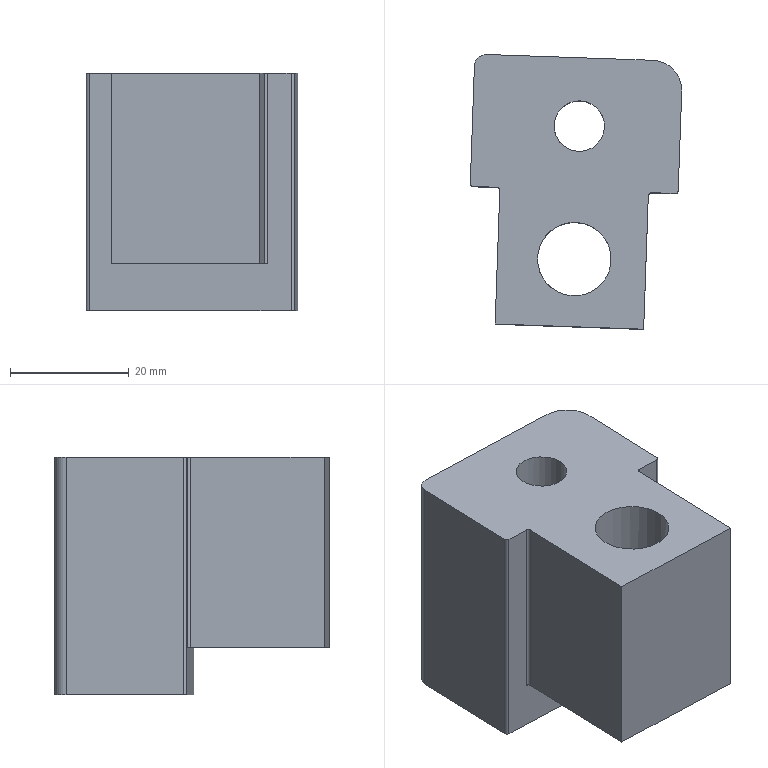Part | NX | features PS-21 2 | 1 solid | 20 faces | box 35.567 x 46.214 x 40 mm | volume 41123 mm3 | plane 11 | cylinder 9 | commonest cylinder face diameters 1 x4 4 x1 8.506 x1 10 x1 12.4 x1 14.5 x1
STEP:
#1=CARTESIAN_POINT('',(3099.937,-917.63,900.716));
#2=VERTEX_POINT('',#1);
#3=CARTESIAN_POINT('',(3100.722,-895.143,900.716));
#4=VERTEX_POINT('',#3);
#5=CARTESIAN_POINT('',(3098.831,-949.294,900.716));
#6=DIRECTION('',(-0.0349,-0.9994,0.));
#7=VECTOR('',#6,1000.);
#8=LINE('',#5,#7);
#9=EDGE_CURVE('',#2,#4,#8,.F.);
#10=ORIENTED_EDGE('',*,*,#9,.T.);
#11=CARTESIAN_POINT('',(3100.722,-895.143,868.716));
#12=VERTEX_POINT('',#11);
#13=CARTESIAN_POINT('',(3100.722,-895.143,868.716));
#14=DIRECTION('',(0.,0.,-1.));
#15=VECTOR('',#14,1000.);
#16=LINE('',#13,#15);
#17=EDGE_CURVE('',#4,#12,#16,.T.);
#18=ORIENTED_EDGE('',*,*,#17,.T.);
#19=CARTESIAN_POINT('',(3099.937,-917.63,868.716));
#20=VERTEX_POINT('',#19);
#21=CARTESIAN_POINT('',(3100.334,-906.255,868.716));
#22=DIRECTION('',(0.0349,0.9994,0.));
#23=VECTOR('',#22,1000.);
#24=LINE('',#21,#23);
#25=EDGE_CURVE('',#20,#12,#24,.T.);
#26=ORIENTED_EDGE('',*,*,#25,.F.);
#27=CARTESIAN_POINT('',(3099.937,-917.63,890.716));
#28=DIRECTION('',(0.,0.,1.));
#29=VECTOR('',#28,1000.);
#30=LINE('',#27,#29);
#31=EDGE_CURVE('',#2,#20,#30,.F.);
#32=ORIENTED_EDGE('',*,*,#31,.F.);
#33=EDGE_LOOP('',(#10,#18,#26,#32));
#34=FACE_BOUND('',#33,.T.);
#35=CARTESIAN_POINT('',(3100.52,-900.918,890.716));
#36=DIRECTION('',(0.9994,-0.0349,0.));
#37=DIRECTION('',(-0.0349,-0.9994,0.));
#38=AXIS2_PLACEMENT_3D('',#35,#36,#37);
#39=PLANE('',#38);
#40=ADVANCED_FACE('',(#34),#39,.F.);
#41=CARTESIAN_POINT('',(3124.922,-918.502,868.716));
#42=VERTEX_POINT('',#41);
#43=CARTESIAN_POINT('',(3109.742,-917.972,868.716));
#44=DIRECTION('',(0.9994,-0.0349,0.));
#45=VECTOR('',#44,1000.);
#46=LINE('',#43,#45);
#47=EDGE_CURVE('',#42,#20,#46,.F.);
#48=ORIENTED_EDGE('',*,*,#47,.F.);
#49=CARTESIAN_POINT('',(3124.922,-918.502,900.716));
#50=VERTEX_POINT('',#49);
#51=CARTESIAN_POINT('',(3124.922,-918.502,862.716));
#52=DIRECTION('',(0.,0.,1.));
#53=VECTOR('',#52,1000.);
#54=LINE('',#51,#53);
#55=EDGE_CURVE('',#50,#42,#54,.F.);
#56=ORIENTED_EDGE('',*,*,#55,.F.);
#57=CARTESIAN_POINT('',(3109.742,-917.972,900.716));
#58=DIRECTION('',(-0.9994,0.0349,0.));
#59=VECTOR('',#58,1000.);
#60=LINE('',#57,#59);
#61=EDGE_CURVE('',#50,#2,#60,.T.);
#62=ORIENTED_EDGE('',*,*,#61,.T.);
#63=ORIENTED_EDGE('',*,*,#31,.T.);
#64=EDGE_LOOP('',(#48,#56,#62,#63));
#65=FACE_BOUND('',#64,.T.);
#66=CARTESIAN_POINT('',(3109.742,-917.972,863.216));
#67=DIRECTION('',(0.0349,0.9994,0.));
#68=DIRECTION('',(-0.9994,0.0349,0.));
#69=AXIS2_PLACEMENT_3D('',#66,#67,#68);
#70=PLANE('',#69);
#71=ADVANCED_FACE('',(#65),#70,.F.);
#72=CARTESIAN_POINT('',(3125.707,-896.016,868.716));
#73=VERTEX_POINT('',#72);
#74=CARTESIAN_POINT('',(3125.319,-907.127,868.716));
#75=DIRECTION('',(0.0349,0.9994,0.));
#76=VECTOR('',#75,1000.);
#77=LINE('',#74,#76);
#78=EDGE_CURVE('',#42,#73,#77,.T.);
#79=ORIENTED_EDGE('',*,*,#78,.T.);
#80=CARTESIAN_POINT('',(3125.707,-896.016,900.716));
#81=VERTEX_POINT('',#80);
#82=CARTESIAN_POINT('',(3125.707,-896.016,862.716));
#83=DIRECTION('',(0.,0.,-1.));
#84=VECTOR('',#83,1000.);
#85=LINE('',#82,#84);
#86=EDGE_CURVE('',#73,#81,#85,.F.);
#87=ORIENTED_EDGE('',*,*,#86,.T.);
#88=CARTESIAN_POINT('',(3123.816,-950.166,900.716));
#89=DIRECTION('',(-0.0349,-0.9994,0.));
#90=VECTOR('',#89,1000.);
#91=LINE('',#88,#90);
#92=EDGE_CURVE('',#50,#81,#91,.F.);
#93=ORIENTED_EDGE('',*,*,#92,.F.);
#94=ORIENTED_EDGE('',*,*,#55,.T.);
#95=EDGE_LOOP('',(#79,#87,#93,#94));
#96=FACE_BOUND('',#95,.T.);
#97=CARTESIAN_POINT('',(3125.54,-900.791,862.716));
#98=DIRECTION('',(0.9994,-0.0349,0.));
#99=DIRECTION('',(-0.0349,-0.9994,0.));
#100=AXIS2_PLACEMENT_3D('',#97,#98,#99);
#101=PLANE('',#100);
#102=ADVANCED_FACE('',(#96),#101,.T.);
#103=CARTESIAN_POINT('',(3107.081,-906.274,868.716));
#104=VERTEX_POINT('',#103);
#105=CARTESIAN_POINT('',(3113.266,-906.707,868.716));
#106=DIRECTION('',(0.,0.,1.));
#107=DIRECTION('',(-0.9976,0.06975,0.));
#108=AXIS2_PLACEMENT_3D('',#105,#106,#107);
#109=CIRCLE('',#108,6.2);
#110=EDGE_CURVE('',#104,#104,#109,.T.);
#111=ORIENTED_EDGE('',*,*,#110,.F.);
#112=EDGE_LOOP('',(#111));
#113=FACE_BOUND('',#112,.T.);
#114=CARTESIAN_POINT('',(3113.266,-900.507,900.716));
#115=VERTEX_POINT('',#114);
#116=CARTESIAN_POINT('',(3113.266,-906.707,900.716));
#117=DIRECTION('',(0.,0.,-1.));
#118=DIRECTION('',(0.,1.,0.));
#119=AXIS2_PLACEMENT_3D('',#116,#117,#118);
#120=CIRCLE('',#119,6.2);
#121=EDGE_CURVE('',#115,#115,#120,.F.);
#122=ORIENTED_EDGE('',*,*,#121,.T.);
#123=EDGE_LOOP('',(#122));
#124=FACE_BOUND('',#123,.T.);
#125=CARTESIAN_POINT('',(3113.266,-906.707,935.716));
#126=DIRECTION('',(0.,0.,-1.));
#127=DIRECTION('',(0.9976,-0.06975,0.));
#128=AXIS2_PLACEMENT_3D('',#125,#126,#127);
#129=CYLINDRICAL_SURFACE('',#128,6.2);
#130=ADVANCED_FACE('',(#113,#124),#129,.F.);
#131=CARTESIAN_POINT('',(3100.24,-894.626,868.716));
#132=VERTEX_POINT('',#131);
#133=CARTESIAN_POINT('',(3126.224,-895.534,868.716));
#134=VERTEX_POINT('',#133);
#135=CARTESIAN_POINT('',(3113.671,-895.095,868.716));
#136=DIRECTION('',(0.9994,-0.0349,0.));
#137=VECTOR('',#136,1000.);
#138=LINE('',#135,#137);
#139=EDGE_CURVE('',#132,#134,#138,.T.);
#140=ORIENTED_EDGE('',*,*,#139,.T.);
#141=CARTESIAN_POINT('',(3126.206,-896.033,868.716));
#142=DIRECTION('',(0.,0.,-1.));
#143=DIRECTION('',(-1.,0.,0.));
#144=AXIS2_PLACEMENT_3D('',#141,#142,#143);
#145=CIRCLE('',#144,0.5);
#146=EDGE_CURVE('',#134,#73,#145,.F.);
#147=ORIENTED_EDGE('',*,*,#146,.T.);
#148=ORIENTED_EDGE('',*,*,#78,.F.);
#149=ORIENTED_EDGE('',*,*,#47,.T.);
#150=ORIENTED_EDGE('',*,*,#25,.T.);
#151=CARTESIAN_POINT('',(3100.222,-895.126,868.716));
#152=DIRECTION('',(0.,0.,-1.));
#153=DIRECTION('',(-1.,0.,0.));
#154=AXIS2_PLACEMENT_3D('',#151,#152,#153);
#155=CIRCLE('',#154,0.5);
#156=EDGE_CURVE('',#12,#132,#155,.F.);
#157=ORIENTED_EDGE('',*,*,#156,.T.);
#158=EDGE_LOOP('',(#140,#147,#148,#149,#150,#157));
#159=FACE_BOUND('',#158,.T.);
#160=ORIENTED_EDGE('',*,*,#110,.T.);
#161=EDGE_LOOP('',(#160));
#162=FACE_BOUND('',#161,.T.);
#163=CARTESIAN_POINT('',(3113.266,-906.707,868.716));
#164=DIRECTION('',(0.,0.,-1.));
#165=DIRECTION('',(-0.0349,-0.9994,0.));
#166=AXIS2_PLACEMENT_3D('',#163,#164,#165);
#167=PLANE('',#166);
#168=ADVANCED_FACE('',(#159,#162),#167,.T.);
#169=ORIENTED_EDGE('',*,*,#121,.F.);
#170=EDGE_LOOP('',(#169));
#171=FACE_BOUND('',#170,.T.);
#172=CARTESIAN_POINT('',(3100.24,-894.626,900.716));
#173=VERTEX_POINT('',#172);
#174=CARTESIAN_POINT('',(3100.222,-895.126,900.716));
#175=DIRECTION('',(0.,0.,-1.));
#176=DIRECTION('',(0.,1.,0.));
#177=AXIS2_PLACEMENT_3D('',#174,#175,#176);
#178=CIRCLE('',#177,0.5);
#179=EDGE_CURVE('',#173,#4,#178,.T.);
#180=ORIENTED_EDGE('',*,*,#179,.T.);
#181=ORIENTED_EDGE('',*,*,#9,.F.);
#182=ORIENTED_EDGE('',*,*,#61,.F.);
#183=ORIENTED_EDGE('',*,*,#92,.T.);
#184=CARTESIAN_POINT('',(3126.224,-895.534,900.716));
#185=VERTEX_POINT('',#184);
#186=CARTESIAN_POINT('',(3126.206,-896.033,900.716));
#187=DIRECTION('',(0.,0.,-1.));
#188=DIRECTION('',(0.,1.,0.));
#189=AXIS2_PLACEMENT_3D('',#186,#187,#188);
#190=CIRCLE('',#189,0.5);
#191=EDGE_CURVE('',#81,#185,#190,.T.);
#192=ORIENTED_EDGE('',*,*,#191,.T.);
#193=CARTESIAN_POINT('',(3130.221,-895.673,900.716));
#194=VERTEX_POINT('',#193);
#195=CARTESIAN_POINT('',(2954.832,-889.549,900.716));
#196=DIRECTION('',(0.9994,-0.0349,0.));
#197=VECTOR('',#196,1000.);
#198=LINE('',#195,#197);
#199=EDGE_CURVE('',#194,#185,#198,.F.);
#200=ORIENTED_EDGE('',*,*,#199,.F.);
#201=CARTESIAN_POINT('',(3130.739,-895.191,900.716));
#202=VERTEX_POINT('',#201);
#203=CARTESIAN_POINT('',(3130.239,-895.173,900.716));
#204=DIRECTION('',(0.,0.,-1.));
#205=DIRECTION('',(0.,1.,0.));
#206=AXIS2_PLACEMENT_3D('',#203,#204,#205);
#207=CIRCLE('',#206,0.5);
#208=EDGE_CURVE('',#194,#202,#207,.F.);
#209=ORIENTED_EDGE('',*,*,#208,.T.);
#210=CARTESIAN_POINT('',(3131.324,-878.438,900.716));
#211=VERTEX_POINT('',#210);
#212=CARTESIAN_POINT('',(3128.813,-950.34,900.716));
#213=DIRECTION('',(-0.0349,-0.9994,0.));
#214=VECTOR('',#213,1000.);
#215=LINE('',#212,#214);
#216=EDGE_CURVE('',#202,#211,#215,.F.);
#217=ORIENTED_EDGE('',*,*,#216,.T.);
#218=CARTESIAN_POINT('',(3126.501,-873.267,900.716));
#219=VERTEX_POINT('',#218);
#220=CARTESIAN_POINT('',(3126.327,-878.264,900.716));
#221=DIRECTION('',(0.,0.,-1.));
#222=DIRECTION('',(0.,1.,0.));
#223=AXIS2_PLACEMENT_3D('',#220,#221,#222);
#224=CIRCLE('',#223,5.);
#225=EDGE_CURVE('',#219,#211,#224,.T.);
#226=ORIENTED_EDGE('',*,*,#225,.F.);
#227=CARTESIAN_POINT('',(3098.518,-872.29,900.716));
#228=VERTEX_POINT('',#227);
#229=CARTESIAN_POINT('',(2955.609,-867.3,900.716));
#230=DIRECTION('',(-0.9994,0.0349,0.));
#231=VECTOR('',#230,1000.);
#232=LINE('',#229,#231);
#233=EDGE_CURVE('',#219,#228,#232,.T.);
#234=ORIENTED_EDGE('',*,*,#233,.T.);
#235=CARTESIAN_POINT('',(3096.45,-874.219,900.716));
#236=VERTEX_POINT('',#235);
#237=CARTESIAN_POINT('',(3098.448,-874.288,900.716));
#238=DIRECTION('',(0.,0.,-1.));
#239=DIRECTION('',(0.,1.,0.));
#240=AXIS2_PLACEMENT_3D('',#237,#238,#239);
#241=CIRCLE('',#240,2.);
#242=EDGE_CURVE('',#236,#228,#241,.T.);
#243=ORIENTED_EDGE('',*,*,#242,.F.);
#244=CARTESIAN_POINT('',(3095.76,-893.97,900.716));
#245=VERTEX_POINT('',#244);
#246=CARTESIAN_POINT('',(3093.834,-949.119,900.716));
#247=DIRECTION('',(-0.0349,-0.9994,0.));
#248=VECTOR('',#247,1000.);
#249=LINE('',#246,#248);
#250=EDGE_CURVE('',#245,#236,#249,.F.);
#251=ORIENTED_EDGE('',*,*,#250,.F.);
#252=CARTESIAN_POINT('',(3096.242,-894.487,900.716));
#253=VERTEX_POINT('',#252);
#254=CARTESIAN_POINT('',(3096.26,-893.987,900.716));
#255=DIRECTION('',(0.,0.,-1.));
#256=DIRECTION('',(0.,1.,0.));
#257=AXIS2_PLACEMENT_3D('',#254,#255,#256);
#258=CIRCLE('',#257,0.5);
#259=EDGE_CURVE('',#245,#253,#258,.F.);
#260=ORIENTED_EDGE('',*,*,#259,.T.);
#261=CARTESIAN_POINT('',(2954.832,-889.549,900.716));
#262=DIRECTION('',(0.9994,-0.0349,0.));
#263=VECTOR('',#262,1000.);
#264=LINE('',#261,#263);
#265=EDGE_CURVE('',#173,#253,#264,.F.);
#266=ORIENTED_EDGE('',*,*,#265,.F.);
#267=EDGE_LOOP('',(#180,#181,#182,#183,#192,#200,#209,#217,#226,#234,#243,#251,#260,#266));
#268=FACE_BOUND('',#267,.T.);
#269=CARTESIAN_POINT('',(3114.107,-880.088,900.716));
#270=VERTEX_POINT('',#269);
#271=CARTESIAN_POINT('',(3114.107,-884.341,900.716));
#272=DIRECTION('',(0.,0.,-1.));
#273=DIRECTION('',(0.,1.,0.));
#274=AXIS2_PLACEMENT_3D('',#271,#272,#273);
#275=CIRCLE('',#274,4.253);
#276=EDGE_CURVE('',#270,#270,#275,.F.);
#277=ORIENTED_EDGE('',*,*,#276,.F.);
#278=EDGE_LOOP('',(#277));
#279=FACE_BOUND('',#278,.T.);
#280=CARTESIAN_POINT('',(2952.924,-944.199,900.716));
#281=DIRECTION('',(0.,0.,1.));
#282=DIRECTION('',(0.9976,-0.06975,0.));
#283=AXIS2_PLACEMENT_3D('',#280,#281,#282);
#284=PLANE('',#283);
#285=ADVANCED_FACE('',(#171,#268,#279),#284,.T.);
#286=ORIENTED_EDGE('',*,*,#179,.F.);
#287=CARTESIAN_POINT('',(3100.24,-894.626,890.716));
#288=DIRECTION('',(0.,0.,-1.));
#289=VECTOR('',#288,1000.);
#290=LINE('',#287,#289);
#291=EDGE_CURVE('',#132,#173,#290,.F.);
#292=ORIENTED_EDGE('',*,*,#291,.F.);
#293=ORIENTED_EDGE('',*,*,#156,.F.);
#294=ORIENTED_EDGE('',*,*,#17,.F.);
#295=EDGE_LOOP('',(#286,#292,#293,#294));
#296=FACE_BOUND('',#295,.T.);
#297=CARTESIAN_POINT('',(3100.222,-895.126,890.716));
#298=DIRECTION('',(0.,0.,1.));
#299=DIRECTION('',(1.,0.,0.));
#300=AXIS2_PLACEMENT_3D('',#297,#298,#299);
#301=CYLINDRICAL_SURFACE('',#300,0.5);
#302=ADVANCED_FACE('',(#296),#301,.F.);
#303=ORIENTED_EDGE('',*,*,#191,.F.);
#304=ORIENTED_EDGE('',*,*,#86,.F.);
#305=ORIENTED_EDGE('',*,*,#146,.F.);
#306=CARTESIAN_POINT('',(3126.224,-895.534,863.216));
#307=DIRECTION('',(0.,0.,-1.));
#308=VECTOR('',#307,1000.);
#309=LINE('',#306,#308);
#310=EDGE_CURVE('',#185,#134,#309,.T.);
#311=ORIENTED_EDGE('',*,*,#310,.F.);
#312=EDGE_LOOP('',(#303,#304,#305,#311));
#313=FACE_BOUND('',#312,.T.);
#314=CARTESIAN_POINT('',(3126.206,-896.033,863.216));
#315=DIRECTION('',(0.,0.,-1.));
#316=DIRECTION('',(-1.,0.,0.));
#317=AXIS2_PLACEMENT_3D('',#314,#315,#316);
#318=CYLINDRICAL_SURFACE('',#317,0.5);
#319=ADVANCED_FACE('',(#313),#318,.F.);
#320=ORIENTED_EDGE('',*,*,#265,.T.);
#321=CARTESIAN_POINT('',(3096.242,-894.487,860.716));
#322=VERTEX_POINT('',#321);
#323=CARTESIAN_POINT('',(3096.242,-894.487,863.216));
#324=DIRECTION('',(0.,0.,1.));
#325=VECTOR('',#324,1000.);
#326=LINE('',#323,#325);
#327=EDGE_CURVE('',#253,#322,#326,.F.);
#328=ORIENTED_EDGE('',*,*,#327,.T.);
#329=CARTESIAN_POINT('',(3130.221,-895.673,860.716));
#330=VERTEX_POINT('',#329);
#331=CARTESIAN_POINT('',(3110.544,-894.986,860.716));
#332=DIRECTION('',(-0.9994,0.0349,0.));
#333=VECTOR('',#332,1000.);
#334=LINE('',#331,#333);
#335=EDGE_CURVE('',#322,#330,#334,.F.);
#336=ORIENTED_EDGE('',*,*,#335,.T.);
#337=CARTESIAN_POINT('',(3130.221,-895.673,890.716));
#338=DIRECTION('',(0.,0.,1.));
#339=VECTOR('',#338,1000.);
#340=LINE('',#337,#339);
#341=EDGE_CURVE('',#330,#194,#340,.T.);
#342=ORIENTED_EDGE('',*,*,#341,.T.);
#343=ORIENTED_EDGE('',*,*,#199,.T.);
#344=ORIENTED_EDGE('',*,*,#310,.T.);
#345=ORIENTED_EDGE('',*,*,#139,.F.);
#346=ORIENTED_EDGE('',*,*,#291,.T.);
#347=EDGE_LOOP('',(#320,#328,#336,#342,#343,#344,#345,#346));
#348=FACE_BOUND('',#347,.T.);
#349=CARTESIAN_POINT('',(3110.544,-894.986,863.216));
#350=DIRECTION('',(0.0349,0.9994,0.));
#351=DIRECTION('',(-0.9994,0.0349,0.));
#352=AXIS2_PLACEMENT_3D('',#349,#350,#351);
#353=PLANE('',#352);
#354=ADVANCED_FACE('',(#348),#353,.F.);
#355=CARTESIAN_POINT('',(3121.357,-884.341,860.716));
#356=VERTEX_POINT('',#355);
#357=CARTESIAN_POINT('',(3114.107,-884.341,860.716));
#358=DIRECTION('',(0.,0.,-1.));
#359=DIRECTION('',(1.,0.,0.));
#360=AXIS2_PLACEMENT_3D('',#357,#358,#359);
#361=CIRCLE('',#360,7.25);
#362=EDGE_CURVE('',#356,#356,#361,.T.);
#363=ORIENTED_EDGE('',*,*,#362,.F.);
#364=EDGE_LOOP('',(#363));
#365=FACE_BOUND('',#364,.T.);
#366=ORIENTED_EDGE('',*,*,#335,.F.);
#367=CARTESIAN_POINT('',(3095.76,-893.97,860.716));
#368=VERTEX_POINT('',#367);
#369=CARTESIAN_POINT('',(3096.26,-893.987,860.716));
#370=DIRECTION('',(0.,0.,-1.));
#371=DIRECTION('',(1.,0.,0.));
#372=AXIS2_PLACEMENT_3D('',#369,#370,#371);
#373=CIRCLE('',#372,0.5);
#374=EDGE_CURVE('',#322,#368,#373,.T.);
#375=ORIENTED_EDGE('',*,*,#374,.T.);
#376=CARTESIAN_POINT('',(3096.45,-874.219,860.716));
#377=VERTEX_POINT('',#376);
#378=CARTESIAN_POINT('',(3101.653,-725.208,860.716));
#379=DIRECTION('',(-0.0349,-0.9994,0.));
#380=VECTOR('',#379,1000.);
#381=LINE('',#378,#380);
#382=EDGE_CURVE('',#368,#377,#381,.F.);
#383=ORIENTED_EDGE('',*,*,#382,.T.);
#384=CARTESIAN_POINT('',(3098.518,-872.29,860.716));
#385=VERTEX_POINT('',#384);
#386=CARTESIAN_POINT('',(3098.448,-874.288,860.716));
#387=DIRECTION('',(0.,0.,-1.));
#388=DIRECTION('',(1.,0.,0.));
#389=AXIS2_PLACEMENT_3D('',#386,#387,#388);
#390=CIRCLE('',#389,2.);
#391=EDGE_CURVE('',#385,#377,#390,.F.);
#392=ORIENTED_EDGE('',*,*,#391,.F.);
#393=CARTESIAN_POINT('',(3126.501,-873.267,860.716));
#394=VERTEX_POINT('',#393);
#395=CARTESIAN_POINT('',(3085.526,-871.836,860.716));
#396=DIRECTION('',(0.9994,-0.0349,0.));
#397=VECTOR('',#396,1000.);
#398=LINE('',#395,#397);
#399=EDGE_CURVE('',#385,#394,#398,.T.);
#400=ORIENTED_EDGE('',*,*,#399,.T.);
#401=CARTESIAN_POINT('',(3131.324,-878.438,860.716));
#402=VERTEX_POINT('',#401);
#403=CARTESIAN_POINT('',(3126.327,-878.264,860.716));
#404=DIRECTION('',(0.,0.,-1.));
#405=DIRECTION('',(1.,0.,0.));
#406=AXIS2_PLACEMENT_3D('',#403,#404,#405);
#407=CIRCLE('',#406,5.);
#408=EDGE_CURVE('',#402,#394,#407,.F.);
#409=ORIENTED_EDGE('',*,*,#408,.F.);
#410=CARTESIAN_POINT('',(3130.739,-895.191,860.716));
#411=VERTEX_POINT('',#410);
#412=CARTESIAN_POINT('',(3136.631,-726.429,860.716));
#413=DIRECTION('',(-0.0349,-0.9994,0.));
#414=VECTOR('',#413,1000.);
#415=LINE('',#412,#414);
#416=EDGE_CURVE('',#411,#402,#415,.F.);
#417=ORIENTED_EDGE('',*,*,#416,.F.);
#418=CARTESIAN_POINT('',(3130.239,-895.173,860.716));
#419=DIRECTION('',(0.,0.,-1.));
#420=DIRECTION('',(1.,0.,0.));
#421=AXIS2_PLACEMENT_3D('',#418,#419,#420);
#422=CIRCLE('',#421,0.5);
#423=EDGE_CURVE('',#411,#330,#422,.T.);
#424=ORIENTED_EDGE('',*,*,#423,.T.);
#425=EDGE_LOOP('',(#366,#375,#383,#392,#400,#409,#417,#424));
#426=FACE_BOUND('',#425,.T.);
#427=CARTESIAN_POINT('',(2870.094,-717.123,860.716));
#428=DIRECTION('',(0.,0.,1.));
#429=DIRECTION('',(0.,-1.,0.));
#430=AXIS2_PLACEMENT_3D('',#427,#428,#429);
#431=PLANE('',#430);
#432=ADVANCED_FACE('',(#365,#426),#431,.F.);
#433=ORIENTED_EDGE('',*,*,#382,.F.);
#434=CARTESIAN_POINT('',(3095.76,-893.97,890.716));
#435=DIRECTION('',(0.,0.,1.));
#436=VECTOR('',#435,1000.);
#437=LINE('',#434,#436);
#438=EDGE_CURVE('',#368,#245,#437,.T.);
#439=ORIENTED_EDGE('',*,*,#438,.T.);
#440=ORIENTED_EDGE('',*,*,#250,.T.);
#441=CARTESIAN_POINT('',(3096.45,-874.219,890.716));
#442=DIRECTION('',(0.,0.,1.));
#443=VECTOR('',#442,1000.);
#444=LINE('',#441,#443);
#445=EDGE_CURVE('',#377,#236,#444,.T.);
#446=ORIENTED_EDGE('',*,*,#445,.F.);
#447=EDGE_LOOP('',(#433,#439,#440,#446));
#448=FACE_BOUND('',#447,.T.);
#449=CARTESIAN_POINT('',(3095.523,-900.744,890.716));
#450=DIRECTION('',(0.9994,-0.0349,0.));
#451=DIRECTION('',(-0.0349,-0.9994,0.));
#452=AXIS2_PLACEMENT_3D('',#449,#450,#451);
#453=PLANE('',#452);
#454=ADVANCED_FACE('',(#448),#453,.F.);
#455=ORIENTED_EDGE('',*,*,#216,.F.);
#456=CARTESIAN_POINT('',(3130.739,-895.191,868.716));
#457=DIRECTION('',(0.,0.,1.));
#458=VECTOR('',#457,1000.);
#459=LINE('',#456,#458);
#460=EDGE_CURVE('',#202,#411,#459,.F.);
#461=ORIENTED_EDGE('',*,*,#460,.T.);
#462=ORIENTED_EDGE('',*,*,#416,.T.);
#463=CARTESIAN_POINT('',(3131.324,-878.438,862.716));
#464=DIRECTION('',(0.,0.,1.));
#465=VECTOR('',#464,1000.);
#466=LINE('',#463,#465);
#467=EDGE_CURVE('',#211,#402,#466,.F.);
#468=ORIENTED_EDGE('',*,*,#467,.F.);
#469=EDGE_LOOP('',(#455,#461,#462,#468));
#470=FACE_BOUND('',#469,.T.);
#471=CARTESIAN_POINT('',(3130.537,-900.966,862.716));
#472=DIRECTION('',(0.9994,-0.0349,0.));
#473=DIRECTION('',(-0.0349,-0.9994,0.));
#474=AXIS2_PLACEMENT_3D('',#471,#472,#473);
#475=PLANE('',#474);
#476=ADVANCED_FACE('',(#470),#475,.T.);
#477=ORIENTED_EDGE('',*,*,#399,.F.);
#478=CARTESIAN_POINT('',(3098.518,-872.29,860.716));
#479=DIRECTION('',(0.,0.,-1.));
#480=VECTOR('',#479,1000.);
#481=LINE('',#478,#480);
#482=EDGE_CURVE('',#228,#385,#481,.T.);
#483=ORIENTED_EDGE('',*,*,#482,.F.);
#484=ORIENTED_EDGE('',*,*,#233,.F.);
#485=CARTESIAN_POINT('',(3126.501,-873.267,935.716));
#486=DIRECTION('',(0.,0.,-1.));
#487=VECTOR('',#486,1000.);
#488=LINE('',#485,#487);
#489=EDGE_CURVE('',#394,#219,#488,.F.);
#490=ORIENTED_EDGE('',*,*,#489,.F.);
#491=EDGE_LOOP('',(#477,#483,#484,#490));
#492=FACE_BOUND('',#491,.T.);
#493=CARTESIAN_POINT('',(3085.526,-871.836,935.716));
#494=DIRECTION('',(-0.0349,-0.9994,0.));
#495=DIRECTION('',(-0.9994,0.0349,0.));
#496=AXIS2_PLACEMENT_3D('',#493,#494,#495);
#497=PLANE('',#496);
#498=ADVANCED_FACE('',(#492),#497,.F.);
#499=ORIENTED_EDGE('',*,*,#242,.T.);
#500=ORIENTED_EDGE('',*,*,#482,.T.);
#501=ORIENTED_EDGE('',*,*,#391,.T.);
#502=ORIENTED_EDGE('',*,*,#445,.T.);
#503=EDGE_LOOP('',(#499,#500,#501,#502));
#504=FACE_BOUND('',#503,.T.);
#505=CARTESIAN_POINT('',(3098.448,-874.288,935.716));
#506=DIRECTION('',(0.,0.,-1.));
#507=DIRECTION('',(-0.9976,0.06975,0.));
#508=AXIS2_PLACEMENT_3D('',#505,#506,#507);
#509=CYLINDRICAL_SURFACE('',#508,2.);
#510=ADVANCED_FACE('',(#504),#509,.T.);
#511=ORIENTED_EDGE('',*,*,#225,.T.);
#512=ORIENTED_EDGE('',*,*,#467,.T.);
#513=ORIENTED_EDGE('',*,*,#408,.T.);
#514=ORIENTED_EDGE('',*,*,#489,.T.);
#515=EDGE_LOOP('',(#511,#512,#513,#514));
#516=FACE_BOUND('',#515,.T.);
#517=CARTESIAN_POINT('',(3126.327,-878.264,862.716));
#518=DIRECTION('',(0.,0.,1.));
#519=DIRECTION('',(0.9976,-0.06975,0.));
#520=AXIS2_PLACEMENT_3D('',#517,#518,#519);
#521=CYLINDRICAL_SURFACE('',#520,5.);
#522=ADVANCED_FACE('',(#516),#521,.T.);
#523=CARTESIAN_POINT('',(3118.35,-884.638,879.716));
#524=VERTEX_POINT('',#523);
#525=CARTESIAN_POINT('',(3114.107,-884.341,879.716));
#526=DIRECTION('',(0.,0.,-1.));
#527=DIRECTION('',(0.9976,-0.06975,0.));
#528=AXIS2_PLACEMENT_3D('',#525,#526,#527);
#529=CIRCLE('',#528,4.253);
#530=EDGE_CURVE('',#524,#524,#529,.T.);
#531=ORIENTED_EDGE('',*,*,#530,.T.);
#532=EDGE_LOOP('',(#531));
#533=FACE_BOUND('',#532,.T.);
#534=ORIENTED_EDGE('',*,*,#276,.T.);
#535=EDGE_LOOP('',(#534));
#536=FACE_BOUND('',#535,.T.);
#537=CARTESIAN_POINT('',(3114.107,-884.341,868.716));
#538=DIRECTION('',(0.,0.,1.));
#539=DIRECTION('',(0.9976,-0.06975,0.));
#540=AXIS2_PLACEMENT_3D('',#537,#538,#539);
#541=CYLINDRICAL_SURFACE('',#540,4.253);
#542=ADVANCED_FACE('',(#533,#536),#541,.F.);
#543=ORIENTED_EDGE('',*,*,#530,.F.);
#544=EDGE_LOOP('',(#543));
#545=FACE_BOUND('',#544,.T.);
#546=CARTESIAN_POINT('',(3121.339,-884.847,879.716));
#547=VERTEX_POINT('',#546);
#548=CARTESIAN_POINT('',(3114.107,-884.341,879.716));
#549=DIRECTION('',(0.,0.,1.));
#550=DIRECTION('',(0.9976,-0.06975,0.));
#551=AXIS2_PLACEMENT_3D('',#548,#549,#550);
#552=CIRCLE('',#551,7.25);
#553=EDGE_CURVE('',#547,#547,#552,.F.);
#554=ORIENTED_EDGE('',*,*,#553,.T.);
#555=EDGE_LOOP('',(#554));
#556=FACE_BOUND('',#555,.T.);
#557=CARTESIAN_POINT('',(3114.107,-884.341,879.716));
#558=DIRECTION('',(0.,0.,1.));
#559=DIRECTION('',(0.9976,-0.06975,0.));
#560=AXIS2_PLACEMENT_3D('',#557,#558,#559);
#561=PLANE('',#560);
#562=ADVANCED_FACE('',(#545,#556),#561,.F.);
#563=ORIENTED_EDGE('',*,*,#553,.F.);
#564=EDGE_LOOP('',(#563));
#565=FACE_BOUND('',#564,.T.);
#566=ORIENTED_EDGE('',*,*,#362,.T.);
#567=EDGE_LOOP('',(#566));
#568=FACE_BOUND('',#567,.T.);
#569=CARTESIAN_POINT('',(3114.107,-884.341,868.716));
#570=DIRECTION('',(0.,0.,1.));
#571=DIRECTION('',(0.9976,-0.06975,0.));
#572=AXIS2_PLACEMENT_3D('',#569,#570,#571);
#573=CYLINDRICAL_SURFACE('',#572,7.25);
#574=ADVANCED_FACE('',(#565,#568),#573,.F.);
#575=ORIENTED_EDGE('',*,*,#423,.F.);
#576=ORIENTED_EDGE('',*,*,#460,.F.);
#577=ORIENTED_EDGE('',*,*,#208,.F.);
#578=ORIENTED_EDGE('',*,*,#341,.F.);
#579=EDGE_LOOP('',(#575,#576,#577,#578));
#580=FACE_BOUND('',#579,.T.);
#581=CARTESIAN_POINT('',(3130.239,-895.173,863.216));
#582=DIRECTION('',(0.,0.,-1.));
#583=DIRECTION('',(-1.,0.,0.));
#584=AXIS2_PLACEMENT_3D('',#581,#582,#583);
#585=CYLINDRICAL_SURFACE('',#584,0.5);
#586=ADVANCED_FACE('',(#580),#585,.T.);
#587=ORIENTED_EDGE('',*,*,#374,.F.);
#588=ORIENTED_EDGE('',*,*,#327,.F.);
#589=ORIENTED_EDGE('',*,*,#259,.F.);
#590=ORIENTED_EDGE('',*,*,#438,.F.);
#591=EDGE_LOOP('',(#587,#588,#589,#590));
#592=FACE_BOUND('',#591,.T.);
#593=CARTESIAN_POINT('',(3096.26,-893.987,890.716));
#594=DIRECTION('',(0.,0.,1.));
#595=DIRECTION('',(1.,0.,0.));
#596=AXIS2_PLACEMENT_3D('',#593,#594,#595);
#597=CYLINDRICAL_SURFACE('',#596,0.5);
#598=ADVANCED_FACE('',(#592),#597,.T.);
#599=CLOSED_SHELL('',(#40,#71,#102,#130,#168,#285,#302,#319,#354,#432,#454,#476,#498,#510,#522,#542,#562,#574,#586,#598));
#600=MANIFOLD_SOLID_BREP('',#599);
#601=(LENGTH_UNIT()NAMED_UNIT(*)SI_UNIT(.MILLI.,.METRE.));
#602=UNCERTAINTY_MEASURE_WITH_UNIT(LENGTH_MEASURE(0.00001),#601,'','');
#603=(NAMED_UNIT(*)PLANE_ANGLE_UNIT()SI_UNIT($,.RADIAN.));
#604=(NAMED_UNIT(*)SI_UNIT($,.STERADIAN.)SOLID_ANGLE_UNIT());
#605=(GEOMETRIC_REPRESENTATION_CONTEXT(3)GLOBAL_UNCERTAINTY_ASSIGNED_CONTEXT((#602))GLOBAL_UNIT_ASSIGNED_CONTEXT((#601,#603,#604))REPRESENTATION_CONTEXT('',''));
#606=ADVANCED_BREP_SHAPE_REPRESENTATION('',(#600),#605);